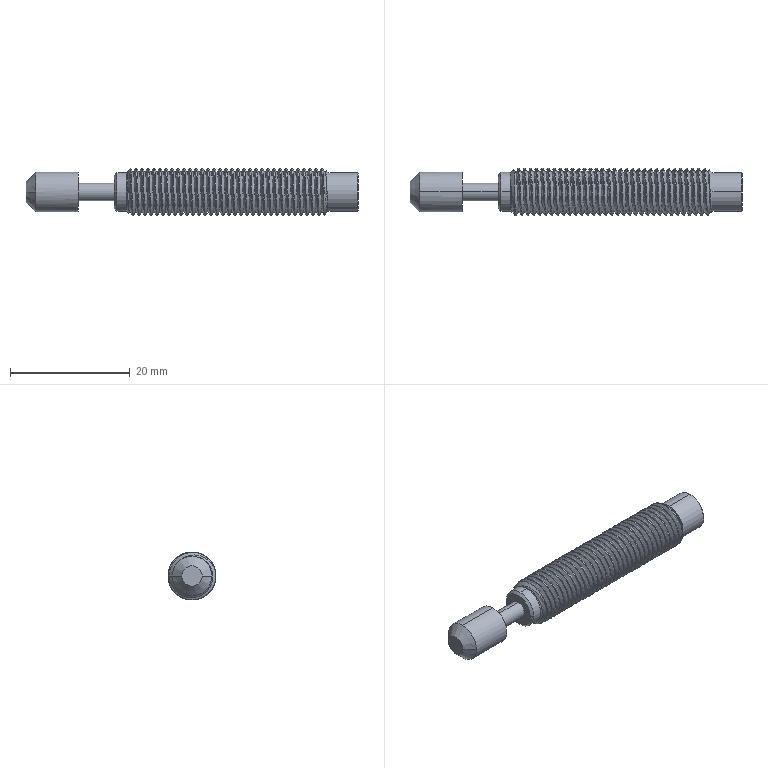Part | STEP file | QA-SKSC0806-1 | 1 solid | 91 faces | box 55.353 x 8 x 8 mm | volume 1947 mm3 | cylinder 73 | cone 12 | plane 4 | spline 2 | commonest cylinder face diameters 8 x65 6.5 x4 2.9 x2 6.6 x2